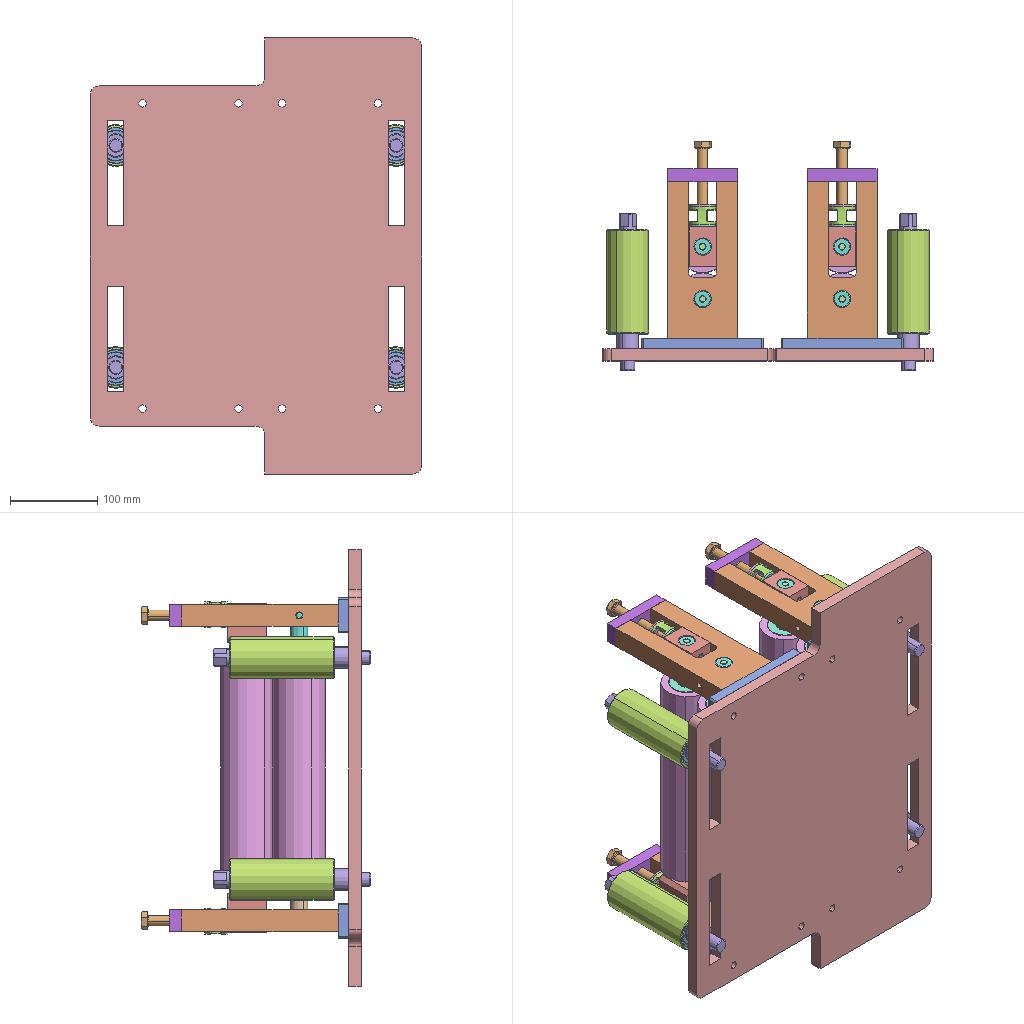Assembly | SolidWorks | 19 different items | 75 placed | box 380 x 263 x 500 mm
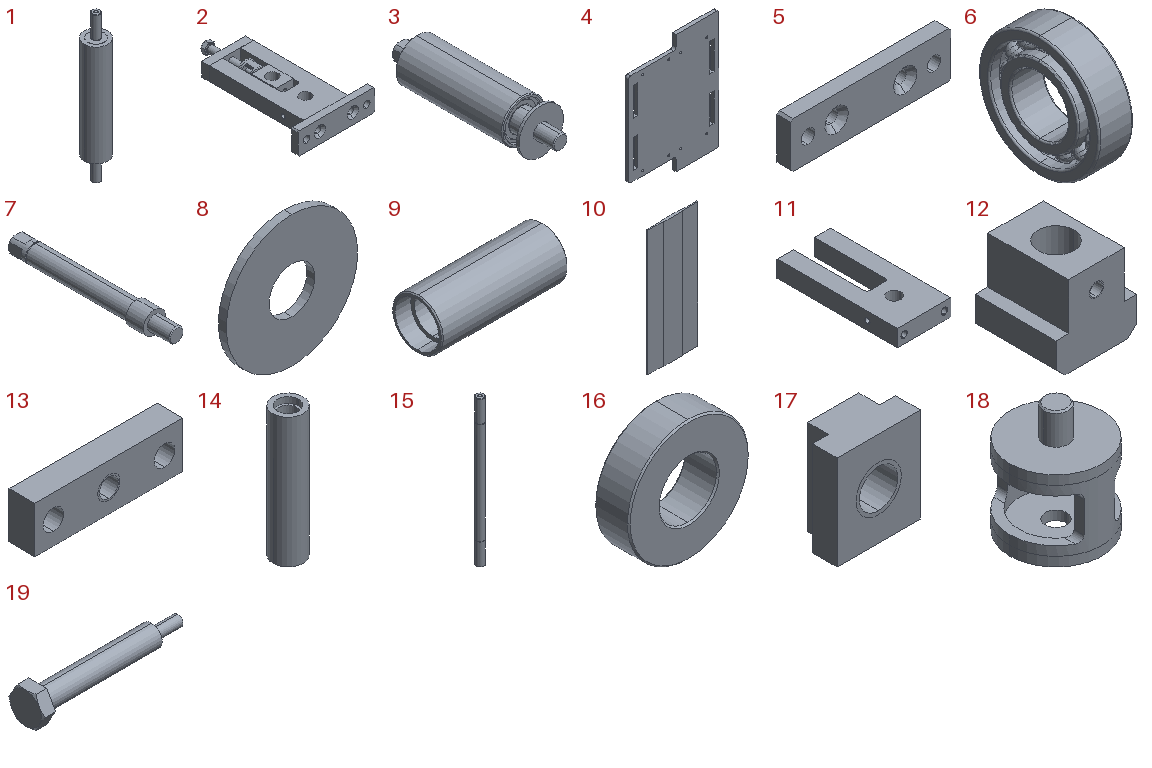Parts list (item | name | quantity | parent item | size | volume | features):
1 | (subassembly) | x4 | - | 60 x 60 x 375 mm | 434095 mm3 | -
2 | (subassembly) | x4 | - | 140 x 238 x 51.5 mm | 422457 mm3 | features AEMSimFeature 1
3 | (subassembly) | x4 | - | 50 x 180 x 50 mm | 169491 mm3 | features AEMSimFeature 1
4 | - | x1 | - | 380 x 14 x 500 mm | 2220724 mm3 | features Fillet 2, ICE 2, Extrusion 1, HoleWzd 1, LPattern 1
5 | - | x4 | in 2 | 140 x 12 x 40 mm | 61151 mm3 | features HoleWzd 2, Chamfer 1, Extrusion 1
6 | - | x8 | in 3 | 12 x 42 x 42 mm | 9468 mm3 | features Revolution 5, CirPattern 2, RefAxis 1, RevCut 1
7 | - | x4 | in 3 | 25 x 180 x 25 mm | 56541 mm3 | features ICE 3, Chamfer 1, RevCut 1, Revolution 1
8 | - | x4 | in 3 | 50 x 3 x 50 mm | 5169 mm3 | features Extrusion 1
9 | - | x4 | in 3 | 120 x 48 x 48 mm | 88845 mm3 | features ICE 4, Chamfer 3, RevCut 1, Revolution 1
10 | - | x1 | - | 200 x 10 x 500 mm | 687500 mm3 | features Extrusion 1, ICE 1
11 | - | x4 | in 2 | - | - | features RefSurface 5, BaseBody 1
12 | - | x4 | in 2 | - | - | features BaseBody 1, RefSurface 1
13 | - | x4 | in 2 | - | - | features BaseBody 1, RefSurface 1
14 | - | x4 | in 1 | 60 x 60 x 260 mm | 474823 mm3 | features BaseBody 1
15 | - | x4 | in 1 | - | - | features BaseBody 3, RefSurface 1
16 | - | x8 | in 1 | 42 x 12 x 42 mm | 12807 mm3 | features BaseBody 1
17 | - | x1 | in 3 | - | - | features BaseBody 1, RefSurface 1
18 | - | x4 | in 2 | 30 x 30 x 36 mm | 6927 mm3 | features ICE 4, HoleWzd 2, Chamfer 1, Extrusion 1, Fillet 1
19 | - | x4 | in 2 | 87.5 x 20.785 x 18 mm | 9848 mm3 | features Chamfer 2, ICE 2, RevCut 2, Revolution 2, Extrusion 1
Mates (type | each side: item.copy, entity, surface, feature):
In the top assembly
Coincident | 4.1 face plane Boss-Extrude1 | assembly face
Coincident | 4.1 face plane Boss-Extrude1 | 5.1 face plane Boss-Extrude1
Coincident | 4.1 face plane Boss-Extrude1 | 5.2 face plane Boss-Extrude1
Concentric | 4.1 face cylinder M10 Tapped Hole1 | 5.2 face cylinder M10 Clearance Hole1 | 2 times
Concentric | 4.1 face cylinder M10 Tapped Hole1 | 5.1 face cylinder M10 Clearance Hole1 | 2 times
Coincident | 4.1 face plane Boss-Extrude1 | 7.1 face plane Revolve1
Coincident | 4.1 face plane Boss-Extrude1 | 7.2 face plane Revolve1
DistanceDim | 10.1 face plane Boss-Extrude1 | 14.1 face plane Input1
DistanceDim | 10.1 face plane Boss-Extrude2 | 4.1 face plane Boss-Extrude1
Width | 4.1 face plane Cut-Extrude2 | 4.1 face plane Cut-Extrude2 | 7.1 face cylinder Revolve1
Width | 4.1 face plane Cut-Extrude2 | 4.1 face plane Cut-Extrude2 | 7.2 face cylinder Revolve1
Concentric | 11.1 edge | 15.1 face cylinder Input24
Concentric | 12.1 face cylinder Input1 | 15.2 face cylinder Input24
Width | 11.1 face plane Input1 | 11.2 face plane Input1 | 15.2 face plane Surface-Input12 | 15.2 face plane Input24
Width | 11.1 face plane Input1 | 11.2 face plane Input1 | 15.1 face plane Surface-Input12 | 15.1 face plane Input24
In subassembly 3
Coincident | 7.3 face plane Revolve1 | 6.1 face plane Revolve1
Concentric | 7.3 face cylinder Revolve1 | 6.1 face cylinder Revolve1
Coincident | 6.1 face plane Revolve1 | 9.1 face plane Cut-Extrude1
Concentric | 7.3 face cylinder Revolve1 | 9.1 face cylinder Cut-Extrude3
Coincident | 6.2 face plane Revolve1 | 9.1 face plane Cut-Extrude2
Concentric | 7.3 face cylinder Revolve1 | 6.2 face cylinder Revolve1
Coincident | 9.1 face plane Revolve1 | 3.1 face
Concentric | 9.1 face cylinder Cut-Extrude2 | 3.1 face
Concentric | 7.3 face cylinder Revolve1 | 3.1 face | 4 times
Coincident | 7.3 face plane Revolve1 | 3.1 face | 2 times
Coincident | 7.3 face plane Revolve1 | 8.1 face plane Boss-Extrude1
Concentric | 7.3 face cylinder Revolve1 | 8.1 face cylinder Boss-Extrude1
DistanceDim | 7.3 face plane Revolve1 | 3.1 face
Concentric | 7.3 face cylinder Revolve1 | 17.1 face
DistanceDim | 17.1 face | 7.3 face plane Revolve1
DistanceDim | 3.1 face | 3.1 face
In subassembly 2
Coincident | 5.3 face plane Boss-Extrude1 | 11.3 face plane Input1
DistanceDim | 5.3 face plane Boss-Extrude1 | 11.3 face plane Input1
Width | 11.3 face plane Input1 | 11.3 face plane Input1 | 5.3 face plane Boss-Extrude1 | 5.3 face plane Boss-Extrude1
Coincident | 11.3 face plane Input1 | 13.1 face plane Input1 | 3 times
DistanceDim | 11.3 face plane Input1 | 12.2 face plane Input1
Coincident | 11.3 face plane Input1 | 12.2 face plane Input1
Coincident | 12.2 face plane Input1 | 18.1 face plane Boss-Extrude2
Concentric | 12.2 face cylinder Input1 | 18.1 face cylinder Boss-Extrude1
Coincident | 18.1 face plane Boss-Extrude3 | 19.1 face plane Cut-Extrude2
Concentric | 13.1 face cylinder Input1 | 19.1 face cylinder Revolve1
DistanceDim | 12.2 face plane Input1 | 11.3 face plane Input1